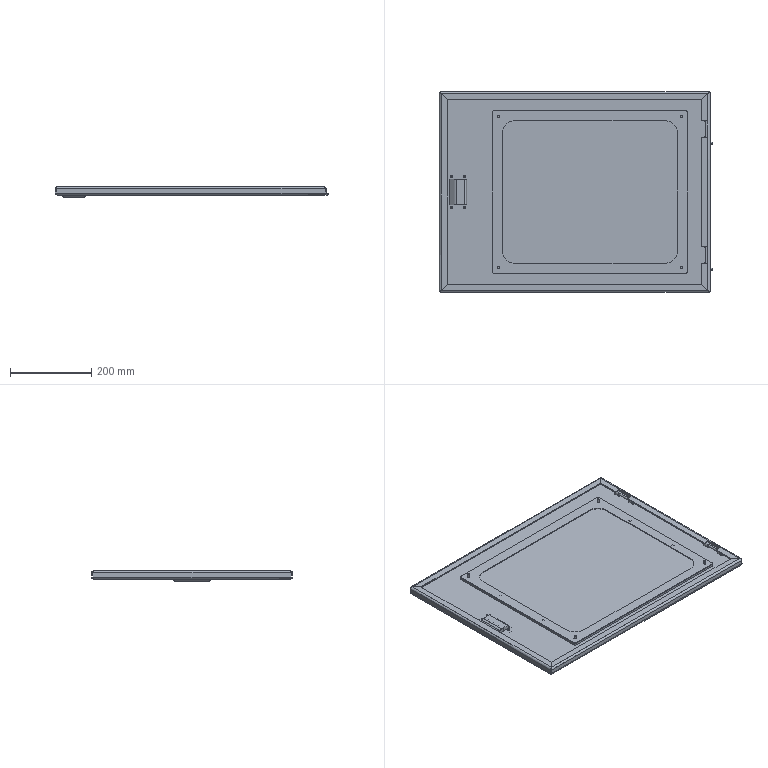Part | SolidWorks | features MirrorCompFeat 1, ReferencePattern 1 | 8 solids | 254 faces | box 670.712 x 493 x 25 mm | volume 1584341 mm3 | plane 133 | cylinder 93 | spline 16 | cone 8 | torus 4 | commonest cylinder face diameters 6 x28 5 x24 10 x16 4 x8 60 x8 20 x4